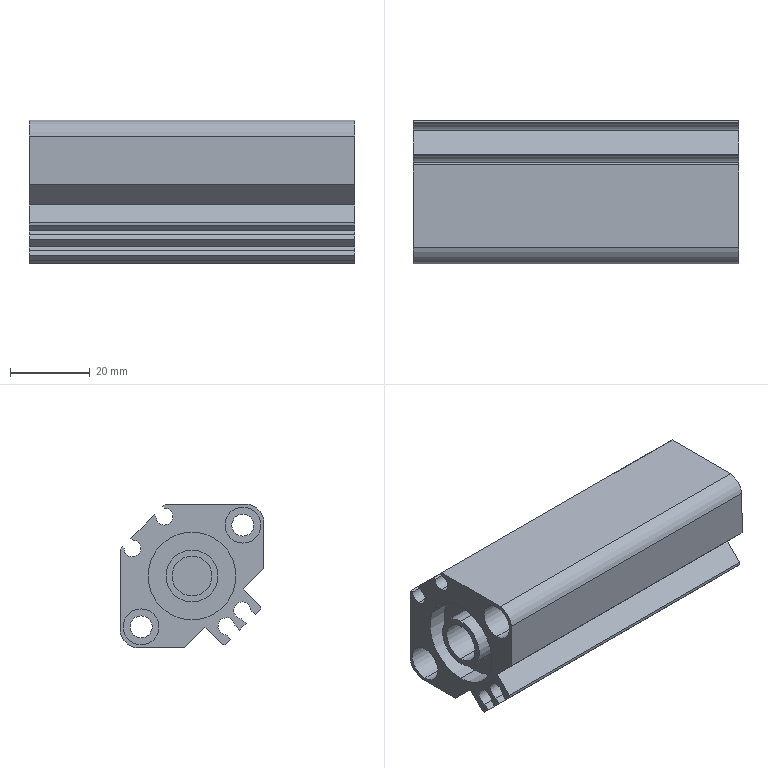Part | SolidWorks | features BaseBody 1 | 1 solid | 79 faces | box 81.5 x 36 x 36 mm | volume 60391 mm3 | cylinder 38 | plane 37 | cone 4 | commonest cylinder face diameters 4.26 x10 9 x8 4.134 x4 5.5 x4 10 x4 22 x4